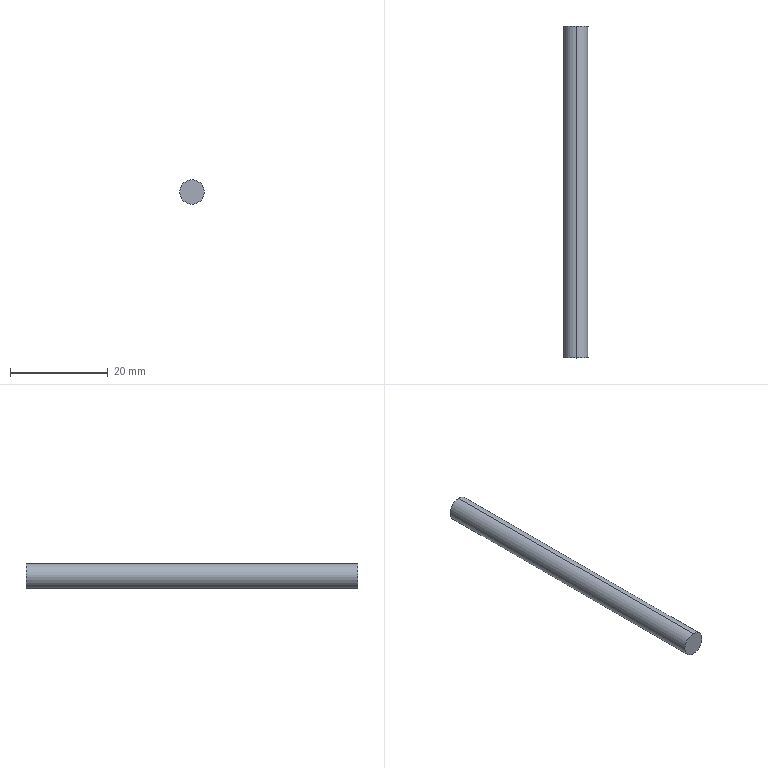Part | STEP file | Rear winding spool | 1 solid | 4 faces | box 5 x 68 x 5 mm | volume 1335 mm3 | cylinder 2 | plane 2 | commonest cylinder face diameters 5 x2
STEP:
#1=CARTESIAN_POINT('',(0.,0.,0.));
#2=DIRECTION('',(0.,0.,1.));
#3=DIRECTION('',(1.,0.,0.));
#4=AXIS2_PLACEMENT_3D('',#1,#2,#3);
#5=CARTESIAN_POINT('',(0.,68.,2.5));
#6=VERTEX_POINT('',#5);
#7=CARTESIAN_POINT('',(0.,68.,-2.5));
#8=VERTEX_POINT('',#7);
#9=CARTESIAN_POINT('',(0.,68.,0.));
#10=DIRECTION('',(0.,1.,0.));
#11=DIRECTION('',(0.,0.,1.));
#12=AXIS2_PLACEMENT_3D('',#9,#10,#11);
#13=CIRCLE('',#12,2.5);
#14=CARTESIAN_POINT('',(0.,68.,0.));
#15=DIRECTION('',(0.,-1.,0.));
#16=DIRECTION('',(0.,0.,-1.));
#17=AXIS2_PLACEMENT_3D('',#14,#15,#16);
#18=CYLINDRICAL_SURFACE('',#17,2.5);
#19=CARTESIAN_POINT('',(3.142,0.));
#20=DIRECTION('',(-1.,0.));
#21=VECTOR('',#20,1.);
#22=LINE('',#19,#21);
#23=(GEOMETRIC_REPRESENTATION_CONTEXT(2)PARAMETRIC_REPRESENTATION_CONTEXT()REPRESENTATION_CONTEXT('',''));
#24=DEFINITIONAL_REPRESENTATION('',(#22),#23);
#25=PCURVE('',#18,#24);
#26=CARTESIAN_POINT('',(0.,68.,0.));
#27=DIRECTION('',(0.,1.,0.));
#28=DIRECTION('',(0.,0.,1.));
#29=AXIS2_PLACEMENT_3D('',#26,#27,#28);
#30=PLANE('',#29);
#31=CARTESIAN_POINT('',(0.,0.));
#32=DIRECTION('',(1.,0.));
#33=AXIS2_PLACEMENT_2D('',#31,#32);
#34=CIRCLE('',#33,2.5);
#35=(GEOMETRIC_REPRESENTATION_CONTEXT(2)PARAMETRIC_REPRESENTATION_CONTEXT()REPRESENTATION_CONTEXT('',''));
#36=DEFINITIONAL_REPRESENTATION('',(#34),#35);
#37=PCURVE('',#30,#36);
#38=SURFACE_CURVE('',#13,(#25,#37),.PCURVE_S1.);
#39=EDGE_CURVE('',#6,#8,#38,.T.);
#40=ORIENTED_EDGE('',*,*,#39,.F.);
#41=CARTESIAN_POINT('',(0.,0.,2.5));
#42=VERTEX_POINT('',#41);
#43=CARTESIAN_POINT('',(0.,68.,2.5));
#44=DIRECTION('',(0.,-1.,0.));
#45=VECTOR('',#44,1.);
#46=LINE('',#43,#45);
#47=CARTESIAN_POINT('',(3.142,0.));
#48=DIRECTION('',(0.,1.));
#49=VECTOR('',#48,1.);
#50=LINE('',#47,#49);
#51=(GEOMETRIC_REPRESENTATION_CONTEXT(2)PARAMETRIC_REPRESENTATION_CONTEXT()REPRESENTATION_CONTEXT('',''));
#52=DEFINITIONAL_REPRESENTATION('',(#50),#51);
#53=PCURVE('',#18,#52);
#54=CARTESIAN_POINT('',(0.,68.,0.));
#55=DIRECTION('',(0.,-1.,0.));
#56=DIRECTION('',(0.,0.,-1.));
#57=AXIS2_PLACEMENT_3D('',#54,#55,#56);
#58=CYLINDRICAL_SURFACE('',#57,2.5);
#59=CARTESIAN_POINT('',(3.142,0.));
#60=DIRECTION('',(0.,1.));
#61=VECTOR('',#60,1.);
#62=LINE('',#59,#61);
#63=(GEOMETRIC_REPRESENTATION_CONTEXT(2)PARAMETRIC_REPRESENTATION_CONTEXT()REPRESENTATION_CONTEXT('',''));
#64=DEFINITIONAL_REPRESENTATION('',(#62),#63);
#65=PCURVE('',#58,#64);
#66=SURFACE_CURVE('',#46,(#53,#65),.PCURVE_S1.);
#67=EDGE_CURVE('',#6,#42,#66,.T.);
#68=ORIENTED_EDGE('',*,*,#67,.T.);
#69=CARTESIAN_POINT('',(0.,0.,-2.5));
#70=VERTEX_POINT('',#69);
#71=CARTESIAN_POINT('',(0.,0.,0.));
#72=DIRECTION('',(0.,1.,0.));
#73=DIRECTION('',(0.,0.,1.));
#74=AXIS2_PLACEMENT_3D('',#71,#72,#73);
#75=CIRCLE('',#74,2.5);
#76=CARTESIAN_POINT('',(3.142,68.));
#77=DIRECTION('',(-1.,0.));
#78=VECTOR('',#77,1.);
#79=LINE('',#76,#78);
#80=(GEOMETRIC_REPRESENTATION_CONTEXT(2)PARAMETRIC_REPRESENTATION_CONTEXT()REPRESENTATION_CONTEXT('',''));
#81=DEFINITIONAL_REPRESENTATION('',(#79),#80);
#82=PCURVE('',#18,#81);
#83=CARTESIAN_POINT('',(0.,0.,0.));
#84=DIRECTION('',(0.,1.,0.));
#85=DIRECTION('',(0.,0.,1.));
#86=AXIS2_PLACEMENT_3D('',#83,#84,#85);
#87=PLANE('',#86);
#88=CARTESIAN_POINT('',(0.,0.));
#89=DIRECTION('',(1.,0.));
#90=AXIS2_PLACEMENT_2D('',#88,#89);
#91=CIRCLE('',#90,2.5);
#92=(GEOMETRIC_REPRESENTATION_CONTEXT(2)PARAMETRIC_REPRESENTATION_CONTEXT()REPRESENTATION_CONTEXT('',''));
#93=DEFINITIONAL_REPRESENTATION('',(#91),#92);
#94=PCURVE('',#87,#93);
#95=SURFACE_CURVE('',#75,(#82,#94),.PCURVE_S1.);
#96=EDGE_CURVE('',#42,#70,#95,.T.);
#97=ORIENTED_EDGE('',*,*,#96,.T.);
#98=CARTESIAN_POINT('',(0.,68.,-2.5));
#99=DIRECTION('',(0.,-1.,0.));
#100=VECTOR('',#99,1.);
#101=LINE('',#98,#100);
#102=CARTESIAN_POINT('',(0.,0.));
#103=DIRECTION('',(0.,1.));
#104=VECTOR('',#103,1.);
#105=LINE('',#102,#104);
#106=(GEOMETRIC_REPRESENTATION_CONTEXT(2)PARAMETRIC_REPRESENTATION_CONTEXT()REPRESENTATION_CONTEXT('',''));
#107=DEFINITIONAL_REPRESENTATION('',(#105),#106);
#108=PCURVE('',#18,#107);
#109=CARTESIAN_POINT('',(6.283,0.));
#110=DIRECTION('',(0.,1.));
#111=VECTOR('',#110,1.);
#112=LINE('',#109,#111);
#113=(GEOMETRIC_REPRESENTATION_CONTEXT(2)PARAMETRIC_REPRESENTATION_CONTEXT()REPRESENTATION_CONTEXT('',''));
#114=DEFINITIONAL_REPRESENTATION('',(#112),#113);
#115=PCURVE('',#58,#114);
#116=SURFACE_CURVE('',#101,(#108,#115),.PCURVE_S1.);
#117=EDGE_CURVE('',#8,#70,#116,.T.);
#118=ORIENTED_EDGE('',*,*,#117,.F.);
#119=EDGE_LOOP('',(#40,#68,#97,#118));
#120=FACE_BOUND('',#119,.T.);
#121=ADVANCED_FACE('',(#120),#18,.T.);
#122=ORIENTED_EDGE('',*,*,#67,.F.);
#123=CARTESIAN_POINT('',(0.,68.,0.));
#124=DIRECTION('',(0.,1.,0.));
#125=DIRECTION('',(0.,0.,1.));
#126=AXIS2_PLACEMENT_3D('',#123,#124,#125);
#127=CIRCLE('',#126,2.5);
#128=CARTESIAN_POINT('',(9.425,0.));
#129=DIRECTION('',(-1.,0.));
#130=VECTOR('',#129,1.);
#131=LINE('',#128,#130);
#132=(GEOMETRIC_REPRESENTATION_CONTEXT(2)PARAMETRIC_REPRESENTATION_CONTEXT()REPRESENTATION_CONTEXT('',''));
#133=DEFINITIONAL_REPRESENTATION('',(#131),#132);
#134=PCURVE('',#58,#133);
#135=CARTESIAN_POINT('',(0.,0.));
#136=DIRECTION('',(1.,0.));
#137=AXIS2_PLACEMENT_2D('',#135,#136);
#138=CIRCLE('',#137,2.5);
#139=(GEOMETRIC_REPRESENTATION_CONTEXT(2)PARAMETRIC_REPRESENTATION_CONTEXT()REPRESENTATION_CONTEXT('',''));
#140=DEFINITIONAL_REPRESENTATION('',(#138),#139);
#141=PCURVE('',#30,#140);
#142=SURFACE_CURVE('',#127,(#134,#141),.PCURVE_S1.);
#143=EDGE_CURVE('',#8,#6,#142,.T.);
#144=ORIENTED_EDGE('',*,*,#143,.F.);
#145=ORIENTED_EDGE('',*,*,#117,.T.);
#146=CARTESIAN_POINT('',(0.,0.,0.));
#147=DIRECTION('',(0.,1.,0.));
#148=DIRECTION('',(0.,0.,1.));
#149=AXIS2_PLACEMENT_3D('',#146,#147,#148);
#150=CIRCLE('',#149,2.5);
#151=CARTESIAN_POINT('',(9.425,68.));
#152=DIRECTION('',(-1.,0.));
#153=VECTOR('',#152,1.);
#154=LINE('',#151,#153);
#155=(GEOMETRIC_REPRESENTATION_CONTEXT(2)PARAMETRIC_REPRESENTATION_CONTEXT()REPRESENTATION_CONTEXT('',''));
#156=DEFINITIONAL_REPRESENTATION('',(#154),#155);
#157=PCURVE('',#58,#156);
#158=CARTESIAN_POINT('',(0.,0.));
#159=DIRECTION('',(1.,0.));
#160=AXIS2_PLACEMENT_2D('',#158,#159);
#161=CIRCLE('',#160,2.5);
#162=(GEOMETRIC_REPRESENTATION_CONTEXT(2)PARAMETRIC_REPRESENTATION_CONTEXT()REPRESENTATION_CONTEXT('',''));
#163=DEFINITIONAL_REPRESENTATION('',(#161),#162);
#164=PCURVE('',#87,#163);
#165=SURFACE_CURVE('',#150,(#157,#164),.PCURVE_S1.);
#166=EDGE_CURVE('',#70,#42,#165,.T.);
#167=ORIENTED_EDGE('',*,*,#166,.T.);
#168=EDGE_LOOP('',(#122,#144,#145,#167));
#169=FACE_BOUND('',#168,.T.);
#170=ADVANCED_FACE('',(#169),#58,.T.);
#171=ORIENTED_EDGE('',*,*,#143,.T.);
#172=ORIENTED_EDGE('',*,*,#39,.T.);
#173=EDGE_LOOP('',(#171,#172));
#174=FACE_BOUND('',#173,.T.);
#175=ADVANCED_FACE('',(#174),#30,.T.);
#176=ORIENTED_EDGE('',*,*,#166,.F.);
#177=ORIENTED_EDGE('',*,*,#96,.F.);
#178=EDGE_LOOP('',(#176,#177));
#179=FACE_BOUND('',#178,.T.);
#180=ADVANCED_FACE('',(#179),#87,.F.);
#181=CLOSED_SHELL('',(#121,#170,#175,#180));
#182=MANIFOLD_SOLID_BREP('',#181);
#183=(LENGTH_UNIT()NAMED_UNIT(*)SI_UNIT(.MILLI.,.METRE.));
#184=UNCERTAINTY_MEASURE_WITH_UNIT(LENGTH_MEASURE(0.0000001),#183,'','');
#185=(NAMED_UNIT(*)PLANE_ANGLE_UNIT()SI_UNIT($,.RADIAN.));
#186=(NAMED_UNIT(*)SI_UNIT($,.STERADIAN.)SOLID_ANGLE_UNIT());
#187=(GEOMETRIC_REPRESENTATION_CONTEXT(3)GLOBAL_UNCERTAINTY_ASSIGNED_CONTEXT((#184))GLOBAL_UNIT_ASSIGNED_CONTEXT((#183,#185,#186))REPRESENTATION_CONTEXT('',''));
#188=ADVANCED_BREP_SHAPE_REPRESENTATION('',(#4,#182),#187);